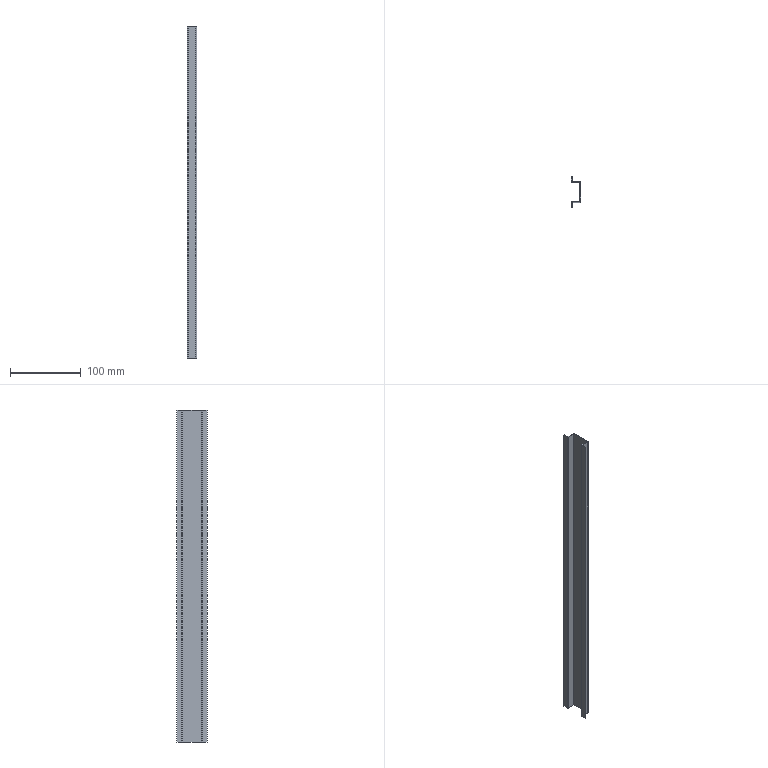Part | STEP file | HESS-408-70-15W-D-6-electrical mounting plate bracket | 1 solid | 22 faces | box 13 x 43 x 470 mm | volume 31006 mm3 | plane 14 | cylinder 8 | commonest cylinder face diameters 0.2 x4 2.2 x4